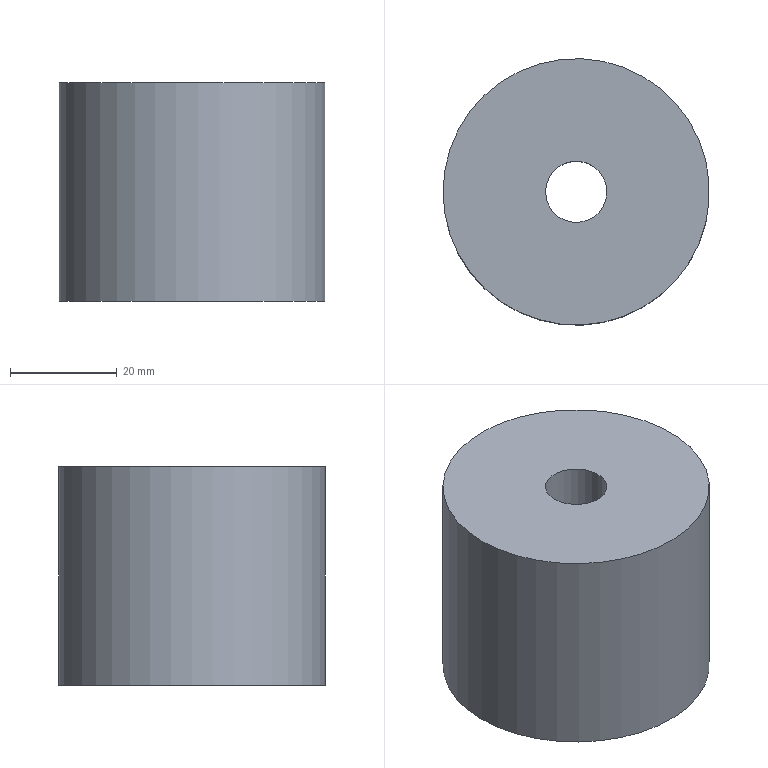Part | NX | features 9 2 | 1 solid | 6 faces | box 50 x 50 x 41 mm | volume 73534 mm3 | cylinder 3 | plane 3 | commonest cylinder face diameters 11.5 x1 18 x1 50 x1
STEP:
#1=CARTESIAN_POINT('',(2852.,-559.,60.));
#2=VERTEX_POINT('',#1);
#3=CARTESIAN_POINT('',(2877.,-559.,60.));
#4=DIRECTION('',(0.,0.,1.));
#5=DIRECTION('',(-1.,0.,0.));
#6=AXIS2_PLACEMENT_3D('',#3,#4,#5);
#7=CIRCLE('',#6,25.);
#8=EDGE_CURVE('',#2,#2,#7,.T.);
#9=ORIENTED_EDGE('',*,*,#8,.T.);
#10=EDGE_LOOP('',(#9));
#11=FACE_BOUND('',#10,.T.);
#12=CARTESIAN_POINT('',(2852.,-559.,101.));
#13=VERTEX_POINT('',#12);
#14=CARTESIAN_POINT('',(2877.,-559.,101.));
#15=DIRECTION('',(0.,0.,-1.));
#16=DIRECTION('',(-1.,0.,0.));
#17=AXIS2_PLACEMENT_3D('',#14,#15,#16);
#18=CIRCLE('',#17,25.);
#19=EDGE_CURVE('',#13,#13,#18,.T.);
#20=ORIENTED_EDGE('',*,*,#19,.T.);
#21=EDGE_LOOP('',(#20));
#22=FACE_BOUND('',#21,.T.);
#23=CARTESIAN_POINT('',(2877.,-559.,20.));
#24=DIRECTION('',(0.,0.,-1.));
#25=DIRECTION('',(-1.,0.,0.));
#26=AXIS2_PLACEMENT_3D('',#23,#24,#25);
#27=CYLINDRICAL_SURFACE('',#26,25.);
#28=ADVANCED_FACE('',(#11,#22),#27,.T.);
#29=CARTESIAN_POINT('',(2882.75,-559.,78.));
#30=VERTEX_POINT('',#29);
#31=CARTESIAN_POINT('',(2877.,-559.,78.));
#32=DIRECTION('',(0.,0.,1.));
#33=DIRECTION('',(1.,0.,0.));
#34=AXIS2_PLACEMENT_3D('',#31,#32,#33);
#35=CIRCLE('',#34,5.75);
#36=EDGE_CURVE('',#30,#30,#35,.T.);
#37=ORIENTED_EDGE('',*,*,#36,.F.);
#38=EDGE_LOOP('',(#37));
#39=FACE_BOUND('',#38,.T.);
#40=CARTESIAN_POINT('',(2882.75,-559.,101.));
#41=VERTEX_POINT('',#40);
#42=CARTESIAN_POINT('',(2877.,-559.,101.));
#43=DIRECTION('',(0.,0.,1.));
#44=DIRECTION('',(1.,0.,0.));
#45=AXIS2_PLACEMENT_3D('',#42,#43,#44);
#46=CIRCLE('',#45,5.75);
#47=EDGE_CURVE('',#41,#41,#46,.T.);
#48=ORIENTED_EDGE('',*,*,#47,.T.);
#49=EDGE_LOOP('',(#48));
#50=FACE_BOUND('',#49,.T.);
#51=CARTESIAN_POINT('',(2877.,-559.,55.));
#52=DIRECTION('',(0.,0.,1.));
#53=DIRECTION('',(1.,0.,0.));
#54=AXIS2_PLACEMENT_3D('',#51,#52,#53);
#55=CYLINDRICAL_SURFACE('',#54,5.75);
#56=ADVANCED_FACE('',(#39,#50),#55,.F.);
#57=CARTESIAN_POINT('',(2868.,-559.,78.));
#58=VERTEX_POINT('',#57);
#59=CARTESIAN_POINT('',(2877.,-559.,78.));
#60=DIRECTION('',(0.,0.,1.));
#61=DIRECTION('',(-1.,0.,0.));
#62=AXIS2_PLACEMENT_3D('',#59,#60,#61);
#63=CIRCLE('',#62,9.);
#64=EDGE_CURVE('',#58,#58,#63,.T.);
#65=ORIENTED_EDGE('',*,*,#64,.T.);
#66=EDGE_LOOP('',(#65));
#67=FACE_BOUND('',#66,.T.);
#68=CARTESIAN_POINT('',(2886.,-559.,60.));
#69=VERTEX_POINT('',#68);
#70=CARTESIAN_POINT('',(2877.,-559.,60.));
#71=DIRECTION('',(0.,0.,-1.));
#72=DIRECTION('',(1.,0.,0.));
#73=AXIS2_PLACEMENT_3D('',#70,#71,#72);
#74=CIRCLE('',#73,9.);
#75=EDGE_CURVE('',#69,#69,#74,.T.);
#76=ORIENTED_EDGE('',*,*,#75,.T.);
#77=EDGE_LOOP('',(#76));
#78=FACE_BOUND('',#77,.T.);
#79=CARTESIAN_POINT('',(2877.,-559.,30.));
#80=DIRECTION('',(0.,0.,1.));
#81=DIRECTION('',(1.,0.,0.));
#82=AXIS2_PLACEMENT_3D('',#79,#80,#81);
#83=CYLINDRICAL_SURFACE('',#82,9.);
#84=ADVANCED_FACE('',(#67,#78),#83,.F.);
#85=ORIENTED_EDGE('',*,*,#36,.T.);
#86=EDGE_LOOP('',(#85));
#87=FACE_BOUND('',#86,.T.);
#88=ORIENTED_EDGE('',*,*,#64,.F.);
#89=EDGE_LOOP('',(#88));
#90=FACE_BOUND('',#89,.T.);
#91=CARTESIAN_POINT('',(2877.,-559.,78.));
#92=DIRECTION('',(0.,0.,1.));
#93=DIRECTION('',(1.,0.,0.));
#94=AXIS2_PLACEMENT_3D('',#91,#92,#93);
#95=PLANE('',#94);
#96=ADVANCED_FACE('',(#87,#90),#95,.F.);
#97=ORIENTED_EDGE('',*,*,#75,.F.);
#98=EDGE_LOOP('',(#97));
#99=FACE_BOUND('',#98,.T.);
#100=ORIENTED_EDGE('',*,*,#8,.F.);
#101=EDGE_LOOP('',(#100));
#102=FACE_BOUND('',#101,.T.);
#103=CARTESIAN_POINT('',(3215.,-814.,60.));
#104=DIRECTION('',(0.,0.,-1.));
#105=DIRECTION('',(-1.,0.,0.));
#106=AXIS2_PLACEMENT_3D('',#103,#104,#105);
#107=PLANE('',#106);
#108=ADVANCED_FACE('',(#99,#102),#107,.T.);
#109=ORIENTED_EDGE('',*,*,#47,.F.);
#110=EDGE_LOOP('',(#109));
#111=FACE_BOUND('',#110,.T.);
#112=ORIENTED_EDGE('',*,*,#19,.F.);
#113=EDGE_LOOP('',(#112));
#114=FACE_BOUND('',#113,.T.);
#115=CARTESIAN_POINT('',(2385.,-938.,101.));
#116=DIRECTION('',(0.,0.,1.));
#117=DIRECTION('',(-1.,0.,0.));
#118=AXIS2_PLACEMENT_3D('',#115,#116,#117);
#119=PLANE('',#118);
#120=ADVANCED_FACE('',(#111,#114),#119,.T.);
#121=CLOSED_SHELL('',(#28,#56,#84,#96,#108,#120));
#122=MANIFOLD_SOLID_BREP('',#121);
#123=(LENGTH_UNIT()NAMED_UNIT(*)SI_UNIT(.MILLI.,.METRE.));
#124=UNCERTAINTY_MEASURE_WITH_UNIT(LENGTH_MEASURE(0.00001),#123,'','');
#125=(NAMED_UNIT(*)PLANE_ANGLE_UNIT()SI_UNIT($,.RADIAN.));
#126=(NAMED_UNIT(*)SI_UNIT($,.STERADIAN.)SOLID_ANGLE_UNIT());
#127=(GEOMETRIC_REPRESENTATION_CONTEXT(3)GLOBAL_UNCERTAINTY_ASSIGNED_CONTEXT((#124))GLOBAL_UNIT_ASSIGNED_CONTEXT((#123,#125,#126))REPRESENTATION_CONTEXT('',''));
#128=ADVANCED_BREP_SHAPE_REPRESENTATION('',(#122),#127);